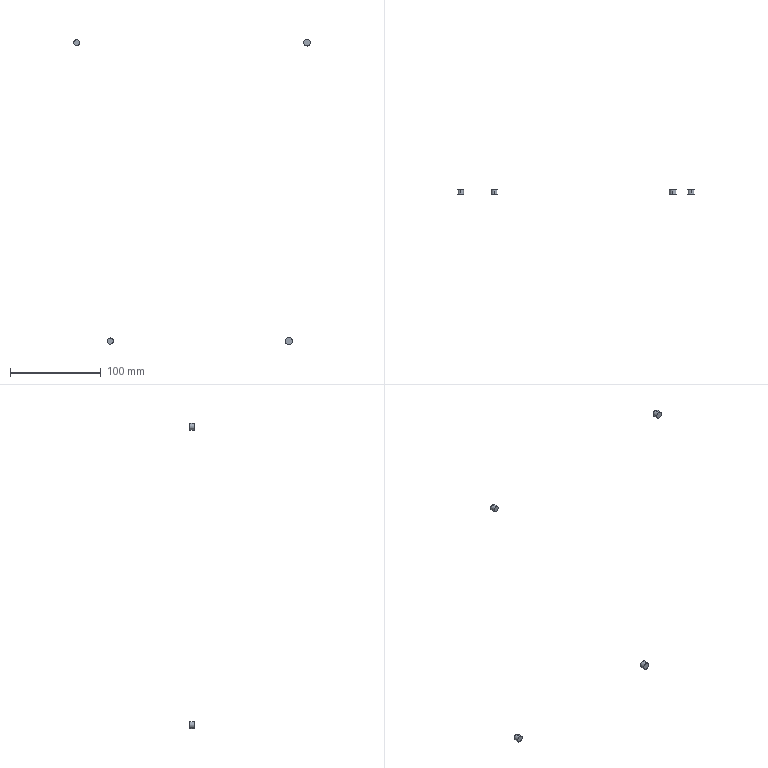Part | STEP file | Pump body | 4 solids | 16 faces | box 260.983 x 5.5 x 336.605 mm | volume 899.272 mm3 | cylinder 8 | plane 8 | commonest cylinder face diameters 6.574 x2 7.014 x2 7.393 x2 7.818 x2
STEP:
#1=CARTESIAN_POINT('',(0.,0.,0.));
#2=DIRECTION('',(0.,0.,1.));
#3=DIRECTION('',(1.,0.,0.));
#4=AXIS2_PLACEMENT_3D('',#1,#2,#3);
#5=CARTESIAN_POINT('',(105.,372.3,-20.091));
#6=VERTEX_POINT('',#5);
#7=CARTESIAN_POINT('',(105.,372.3,-27.909));
#8=VERTEX_POINT('',#7);
#9=CARTESIAN_POINT('',(105.,372.3,-24.));
#10=DIRECTION('',(0.,1.,0.));
#11=DIRECTION('',(0.,0.,1.));
#12=AXIS2_PLACEMENT_3D('',#9,#10,#11);
#13=CIRCLE('',#12,3.909);
#14=CARTESIAN_POINT('',(105.,372.3,-24.));
#15=DIRECTION('',(0.,1.,0.));
#16=DIRECTION('',(0.,0.,1.));
#17=AXIS2_PLACEMENT_3D('',#14,#15,#16);
#18=CYLINDRICAL_SURFACE('',#17,3.909);
#19=CARTESIAN_POINT('',(0.,0.));
#20=DIRECTION('',(1.,0.));
#21=VECTOR('',#20,1.);
#22=LINE('',#19,#21);
#23=(GEOMETRIC_REPRESENTATION_CONTEXT(2)PARAMETRIC_REPRESENTATION_CONTEXT()REPRESENTATION_CONTEXT('',''));
#24=DEFINITIONAL_REPRESENTATION('',(#22),#23);
#25=PCURVE('',#18,#24);
#26=CARTESIAN_POINT('',(105.,372.3,-24.));
#27=DIRECTION('',(0.,1.,0.));
#28=DIRECTION('',(0.,0.,1.));
#29=AXIS2_PLACEMENT_3D('',#26,#27,#28);
#30=PLANE('',#29);
#31=CARTESIAN_POINT('',(0.,0.));
#32=DIRECTION('',(1.,0.));
#33=AXIS2_PLACEMENT_2D('',#31,#32);
#34=CIRCLE('',#33,3.909);
#35=(GEOMETRIC_REPRESENTATION_CONTEXT(2)PARAMETRIC_REPRESENTATION_CONTEXT()REPRESENTATION_CONTEXT('',''));
#36=DEFINITIONAL_REPRESENTATION('',(#34),#35);
#37=PCURVE('',#30,#36);
#38=SURFACE_CURVE('',#13,(#25,#37),.PCURVE_S1.);
#39=EDGE_CURVE('',#6,#8,#38,.T.);
#40=ORIENTED_EDGE('',*,*,#39,.T.);
#41=CARTESIAN_POINT('',(105.,377.8,-27.909));
#42=VERTEX_POINT('',#41);
#43=CARTESIAN_POINT('',(105.,372.3,-27.909));
#44=DIRECTION('',(0.,1.,0.));
#45=VECTOR('',#44,1.);
#46=LINE('',#43,#45);
#47=CARTESIAN_POINT('',(3.142,0.));
#48=DIRECTION('',(0.,1.));
#49=VECTOR('',#48,1.);
#50=LINE('',#47,#49);
#51=(GEOMETRIC_REPRESENTATION_CONTEXT(2)PARAMETRIC_REPRESENTATION_CONTEXT()REPRESENTATION_CONTEXT('',''));
#52=DEFINITIONAL_REPRESENTATION('',(#50),#51);
#53=PCURVE('',#18,#52);
#54=CARTESIAN_POINT('',(105.,372.3,-24.));
#55=DIRECTION('',(0.,1.,0.));
#56=DIRECTION('',(0.,0.,1.));
#57=AXIS2_PLACEMENT_3D('',#54,#55,#56);
#58=CYLINDRICAL_SURFACE('',#57,3.909);
#59=CARTESIAN_POINT('',(3.142,0.));
#60=DIRECTION('',(0.,1.));
#61=VECTOR('',#60,1.);
#62=LINE('',#59,#61);
#63=(GEOMETRIC_REPRESENTATION_CONTEXT(2)PARAMETRIC_REPRESENTATION_CONTEXT()REPRESENTATION_CONTEXT('',''));
#64=DEFINITIONAL_REPRESENTATION('',(#62),#63);
#65=PCURVE('',#58,#64);
#66=SURFACE_CURVE('',#46,(#53,#65),.PCURVE_S1.);
#67=EDGE_CURVE('',#8,#42,#66,.T.);
#68=ORIENTED_EDGE('',*,*,#67,.T.);
#69=CARTESIAN_POINT('',(105.,377.8,-20.091));
#70=VERTEX_POINT('',#69);
#71=CARTESIAN_POINT('',(105.,377.8,-24.));
#72=DIRECTION('',(0.,1.,0.));
#73=DIRECTION('',(0.,0.,1.));
#74=AXIS2_PLACEMENT_3D('',#71,#72,#73);
#75=CIRCLE('',#74,3.909);
#76=CARTESIAN_POINT('',(0.,5.5));
#77=DIRECTION('',(1.,0.));
#78=VECTOR('',#77,1.);
#79=LINE('',#76,#78);
#80=(GEOMETRIC_REPRESENTATION_CONTEXT(2)PARAMETRIC_REPRESENTATION_CONTEXT()REPRESENTATION_CONTEXT('',''));
#81=DEFINITIONAL_REPRESENTATION('',(#79),#80);
#82=PCURVE('',#18,#81);
#83=CARTESIAN_POINT('',(105.,377.8,-24.));
#84=DIRECTION('',(0.,1.,0.));
#85=DIRECTION('',(0.,0.,1.));
#86=AXIS2_PLACEMENT_3D('',#83,#84,#85);
#87=PLANE('',#86);
#88=CARTESIAN_POINT('',(0.,0.));
#89=DIRECTION('',(1.,0.));
#90=AXIS2_PLACEMENT_2D('',#88,#89);
#91=CIRCLE('',#90,3.909);
#92=(GEOMETRIC_REPRESENTATION_CONTEXT(2)PARAMETRIC_REPRESENTATION_CONTEXT()REPRESENTATION_CONTEXT('',''));
#93=DEFINITIONAL_REPRESENTATION('',(#91),#92);
#94=PCURVE('',#87,#93);
#95=SURFACE_CURVE('',#75,(#82,#94),.PCURVE_S1.);
#96=EDGE_CURVE('',#70,#42,#95,.T.);
#97=ORIENTED_EDGE('',*,*,#96,.F.);
#98=CARTESIAN_POINT('',(105.,372.3,-20.091));
#99=DIRECTION('',(0.,1.,0.));
#100=VECTOR('',#99,1.);
#101=LINE('',#98,#100);
#102=CARTESIAN_POINT('',(0.,0.));
#103=DIRECTION('',(0.,1.));
#104=VECTOR('',#103,1.);
#105=LINE('',#102,#104);
#106=(GEOMETRIC_REPRESENTATION_CONTEXT(2)PARAMETRIC_REPRESENTATION_CONTEXT()REPRESENTATION_CONTEXT('',''));
#107=DEFINITIONAL_REPRESENTATION('',(#105),#106);
#108=PCURVE('',#18,#107);
#109=CARTESIAN_POINT('',(6.283,0.));
#110=DIRECTION('',(0.,1.));
#111=VECTOR('',#110,1.);
#112=LINE('',#109,#111);
#113=(GEOMETRIC_REPRESENTATION_CONTEXT(2)PARAMETRIC_REPRESENTATION_CONTEXT()REPRESENTATION_CONTEXT('',''));
#114=DEFINITIONAL_REPRESENTATION('',(#112),#113);
#115=PCURVE('',#58,#114);
#116=SURFACE_CURVE('',#101,(#108,#115),.PCURVE_S1.);
#117=EDGE_CURVE('',#6,#70,#116,.T.);
#118=ORIENTED_EDGE('',*,*,#117,.F.);
#119=EDGE_LOOP('',(#40,#68,#97,#118));
#120=FACE_BOUND('',#119,.T.);
#121=ADVANCED_FACE('',(#120),#18,.T.);
#122=ORIENTED_EDGE('',*,*,#67,.F.);
#123=CARTESIAN_POINT('',(105.,372.3,-24.));
#124=DIRECTION('',(0.,1.,0.));
#125=DIRECTION('',(0.,0.,1.));
#126=AXIS2_PLACEMENT_3D('',#123,#124,#125);
#127=CIRCLE('',#126,3.909);
#128=CARTESIAN_POINT('',(0.,0.));
#129=DIRECTION('',(1.,0.));
#130=VECTOR('',#129,1.);
#131=LINE('',#128,#130);
#132=(GEOMETRIC_REPRESENTATION_CONTEXT(2)PARAMETRIC_REPRESENTATION_CONTEXT()REPRESENTATION_CONTEXT('',''));
#133=DEFINITIONAL_REPRESENTATION('',(#131),#132);
#134=PCURVE('',#58,#133);
#135=CARTESIAN_POINT('',(0.,0.));
#136=DIRECTION('',(1.,0.));
#137=AXIS2_PLACEMENT_2D('',#135,#136);
#138=CIRCLE('',#137,3.909);
#139=(GEOMETRIC_REPRESENTATION_CONTEXT(2)PARAMETRIC_REPRESENTATION_CONTEXT()REPRESENTATION_CONTEXT('',''));
#140=DEFINITIONAL_REPRESENTATION('',(#138),#139);
#141=PCURVE('',#30,#140);
#142=SURFACE_CURVE('',#127,(#134,#141),.PCURVE_S1.);
#143=EDGE_CURVE('',#8,#6,#142,.T.);
#144=ORIENTED_EDGE('',*,*,#143,.T.);
#145=ORIENTED_EDGE('',*,*,#117,.T.);
#146=CARTESIAN_POINT('',(105.,377.8,-24.));
#147=DIRECTION('',(0.,1.,0.));
#148=DIRECTION('',(0.,0.,1.));
#149=AXIS2_PLACEMENT_3D('',#146,#147,#148);
#150=CIRCLE('',#149,3.909);
#151=CARTESIAN_POINT('',(0.,5.5));
#152=DIRECTION('',(1.,0.));
#153=VECTOR('',#152,1.);
#154=LINE('',#151,#153);
#155=(GEOMETRIC_REPRESENTATION_CONTEXT(2)PARAMETRIC_REPRESENTATION_CONTEXT()REPRESENTATION_CONTEXT('',''));
#156=DEFINITIONAL_REPRESENTATION('',(#154),#155);
#157=PCURVE('',#58,#156);
#158=CARTESIAN_POINT('',(0.,0.));
#159=DIRECTION('',(1.,0.));
#160=AXIS2_PLACEMENT_2D('',#158,#159);
#161=CIRCLE('',#160,3.909);
#162=(GEOMETRIC_REPRESENTATION_CONTEXT(2)PARAMETRIC_REPRESENTATION_CONTEXT()REPRESENTATION_CONTEXT('',''));
#163=DEFINITIONAL_REPRESENTATION('',(#161),#162);
#164=PCURVE('',#87,#163);
#165=SURFACE_CURVE('',#150,(#157,#164),.PCURVE_S1.);
#166=EDGE_CURVE('',#42,#70,#165,.T.);
#167=ORIENTED_EDGE('',*,*,#166,.F.);
#168=EDGE_LOOP('',(#122,#144,#145,#167));
#169=FACE_BOUND('',#168,.T.);
#170=ADVANCED_FACE('',(#169),#58,.T.);
#171=ORIENTED_EDGE('',*,*,#39,.F.);
#172=ORIENTED_EDGE('',*,*,#143,.F.);
#173=EDGE_LOOP('',(#171,#172));
#174=FACE_BOUND('',#173,.T.);
#175=ADVANCED_FACE('',(#174),#30,.F.);
#176=ORIENTED_EDGE('',*,*,#96,.T.);
#177=ORIENTED_EDGE('',*,*,#166,.T.);
#178=EDGE_LOOP('',(#176,#177));
#179=FACE_BOUND('',#178,.T.);
#180=ADVANCED_FACE('',(#179),#87,.T.);
#181=CLOSED_SHELL('',(#121,#170,#175,#180));
#182=MANIFOLD_SOLID_BREP('',#181);
#183=CARTESIAN_POINT('',(-92.,372.3,-20.493));
#184=VERTEX_POINT('',#183);
#185=CARTESIAN_POINT('',(-92.,372.3,-27.507));
#186=VERTEX_POINT('',#185);
#187=CARTESIAN_POINT('',(-92.,372.3,-24.));
#188=DIRECTION('',(0.,1.,0.));
#189=DIRECTION('',(0.,0.,1.));
#190=AXIS2_PLACEMENT_3D('',#187,#188,#189);
#191=CIRCLE('',#190,3.507);
#192=CARTESIAN_POINT('',(-92.,372.3,-24.));
#193=DIRECTION('',(0.,1.,0.));
#194=DIRECTION('',(0.,0.,1.));
#195=AXIS2_PLACEMENT_3D('',#192,#193,#194);
#196=CYLINDRICAL_SURFACE('',#195,3.507);
#197=CARTESIAN_POINT('',(0.,0.));
#198=DIRECTION('',(1.,0.));
#199=VECTOR('',#198,1.);
#200=LINE('',#197,#199);
#201=(GEOMETRIC_REPRESENTATION_CONTEXT(2)PARAMETRIC_REPRESENTATION_CONTEXT()REPRESENTATION_CONTEXT('',''));
#202=DEFINITIONAL_REPRESENTATION('',(#200),#201);
#203=PCURVE('',#196,#202);
#204=CARTESIAN_POINT('',(-92.,372.3,-24.));
#205=DIRECTION('',(0.,1.,0.));
#206=DIRECTION('',(0.,0.,1.));
#207=AXIS2_PLACEMENT_3D('',#204,#205,#206);
#208=PLANE('',#207);
#209=CARTESIAN_POINT('',(0.,0.));
#210=DIRECTION('',(1.,0.));
#211=AXIS2_PLACEMENT_2D('',#209,#210);
#212=CIRCLE('',#211,3.507);
#213=(GEOMETRIC_REPRESENTATION_CONTEXT(2)PARAMETRIC_REPRESENTATION_CONTEXT()REPRESENTATION_CONTEXT('',''));
#214=DEFINITIONAL_REPRESENTATION('',(#212),#213);
#215=PCURVE('',#208,#214);
#216=SURFACE_CURVE('',#191,(#203,#215),.PCURVE_S1.);
#217=EDGE_CURVE('',#184,#186,#216,.T.);
#218=ORIENTED_EDGE('',*,*,#217,.T.);
#219=CARTESIAN_POINT('',(-92.,377.8,-27.507));
#220=VERTEX_POINT('',#219);
#221=CARTESIAN_POINT('',(-92.,372.3,-27.507));
#222=DIRECTION('',(0.,1.,0.));
#223=VECTOR('',#222,1.);
#224=LINE('',#221,#223);
#225=CARTESIAN_POINT('',(3.142,0.));
#226=DIRECTION('',(0.,1.));
#227=VECTOR('',#226,1.);
#228=LINE('',#225,#227);
#229=(GEOMETRIC_REPRESENTATION_CONTEXT(2)PARAMETRIC_REPRESENTATION_CONTEXT()REPRESENTATION_CONTEXT('',''));
#230=DEFINITIONAL_REPRESENTATION('',(#228),#229);
#231=PCURVE('',#196,#230);
#232=CARTESIAN_POINT('',(-92.,372.3,-24.));
#233=DIRECTION('',(0.,1.,0.));
#234=DIRECTION('',(0.,0.,1.));
#235=AXIS2_PLACEMENT_3D('',#232,#233,#234);
#236=CYLINDRICAL_SURFACE('',#235,3.507);
#237=CARTESIAN_POINT('',(3.142,0.));
#238=DIRECTION('',(0.,1.));
#239=VECTOR('',#238,1.);
#240=LINE('',#237,#239);
#241=(GEOMETRIC_REPRESENTATION_CONTEXT(2)PARAMETRIC_REPRESENTATION_CONTEXT()REPRESENTATION_CONTEXT('',''));
#242=DEFINITIONAL_REPRESENTATION('',(#240),#241);
#243=PCURVE('',#236,#242);
#244=SURFACE_CURVE('',#224,(#231,#243),.PCURVE_S1.);
#245=EDGE_CURVE('',#186,#220,#244,.T.);
#246=ORIENTED_EDGE('',*,*,#245,.T.);
#247=CARTESIAN_POINT('',(-92.,377.8,-20.493));
#248=VERTEX_POINT('',#247);
#249=CARTESIAN_POINT('',(-92.,377.8,-24.));
#250=DIRECTION('',(0.,1.,0.));
#251=DIRECTION('',(0.,0.,1.));
#252=AXIS2_PLACEMENT_3D('',#249,#250,#251);
#253=CIRCLE('',#252,3.507);
#254=CARTESIAN_POINT('',(0.,5.5));
#255=DIRECTION('',(1.,0.));
#256=VECTOR('',#255,1.);
#257=LINE('',#254,#256);
#258=(GEOMETRIC_REPRESENTATION_CONTEXT(2)PARAMETRIC_REPRESENTATION_CONTEXT()REPRESENTATION_CONTEXT('',''));
#259=DEFINITIONAL_REPRESENTATION('',(#257),#258);
#260=PCURVE('',#196,#259);
#261=CARTESIAN_POINT('',(-92.,377.8,-24.));
#262=DIRECTION('',(0.,1.,0.));
#263=DIRECTION('',(0.,0.,1.));
#264=AXIS2_PLACEMENT_3D('',#261,#262,#263);
#265=PLANE('',#264);
#266=CARTESIAN_POINT('',(0.,0.));
#267=DIRECTION('',(1.,0.));
#268=AXIS2_PLACEMENT_2D('',#266,#267);
#269=CIRCLE('',#268,3.507);
#270=(GEOMETRIC_REPRESENTATION_CONTEXT(2)PARAMETRIC_REPRESENTATION_CONTEXT()REPRESENTATION_CONTEXT('',''));
#271=DEFINITIONAL_REPRESENTATION('',(#269),#270);
#272=PCURVE('',#265,#271);
#273=SURFACE_CURVE('',#253,(#260,#272),.PCURVE_S1.);
#274=EDGE_CURVE('',#248,#220,#273,.T.);
#275=ORIENTED_EDGE('',*,*,#274,.F.);
#276=CARTESIAN_POINT('',(-92.,372.3,-20.493));
#277=DIRECTION('',(0.,1.,0.));
#278=VECTOR('',#277,1.);
#279=LINE('',#276,#278);
#280=CARTESIAN_POINT('',(0.,0.));
#281=DIRECTION('',(0.,1.));
#282=VECTOR('',#281,1.);
#283=LINE('',#280,#282);
#284=(GEOMETRIC_REPRESENTATION_CONTEXT(2)PARAMETRIC_REPRESENTATION_CONTEXT()REPRESENTATION_CONTEXT('',''));
#285=DEFINITIONAL_REPRESENTATION('',(#283),#284);
#286=PCURVE('',#196,#285);
#287=CARTESIAN_POINT('',(6.283,0.));
#288=DIRECTION('',(0.,1.));
#289=VECTOR('',#288,1.);
#290=LINE('',#287,#289);
#291=(GEOMETRIC_REPRESENTATION_CONTEXT(2)PARAMETRIC_REPRESENTATION_CONTEXT()REPRESENTATION_CONTEXT('',''));
#292=DEFINITIONAL_REPRESENTATION('',(#290),#291);
#293=PCURVE('',#236,#292);
#294=SURFACE_CURVE('',#279,(#286,#293),.PCURVE_S1.);
#295=EDGE_CURVE('',#184,#248,#294,.T.);
#296=ORIENTED_EDGE('',*,*,#295,.F.);
#297=EDGE_LOOP('',(#218,#246,#275,#296));
#298=FACE_BOUND('',#297,.T.);
#299=ADVANCED_FACE('',(#298),#196,.T.);
#300=ORIENTED_EDGE('',*,*,#245,.F.);
#301=CARTESIAN_POINT('',(-92.,372.3,-24.));
#302=DIRECTION('',(0.,1.,0.));
#303=DIRECTION('',(0.,0.,1.));
#304=AXIS2_PLACEMENT_3D('',#301,#302,#303);
#305=CIRCLE('',#304,3.507);
#306=CARTESIAN_POINT('',(0.,0.));
#307=DIRECTION('',(1.,0.));
#308=VECTOR('',#307,1.);
#309=LINE('',#306,#308);
#310=(GEOMETRIC_REPRESENTATION_CONTEXT(2)PARAMETRIC_REPRESENTATION_CONTEXT()REPRESENTATION_CONTEXT('',''));
#311=DEFINITIONAL_REPRESENTATION('',(#309),#310);
#312=PCURVE('',#236,#311);
#313=CARTESIAN_POINT('',(0.,0.));
#314=DIRECTION('',(1.,0.));
#315=AXIS2_PLACEMENT_2D('',#313,#314);
#316=CIRCLE('',#315,3.507);
#317=(GEOMETRIC_REPRESENTATION_CONTEXT(2)PARAMETRIC_REPRESENTATION_CONTEXT()REPRESENTATION_CONTEXT('',''));
#318=DEFINITIONAL_REPRESENTATION('',(#316),#317);
#319=PCURVE('',#208,#318);
#320=SURFACE_CURVE('',#305,(#312,#319),.PCURVE_S1.);
#321=EDGE_CURVE('',#186,#184,#320,.T.);
#322=ORIENTED_EDGE('',*,*,#321,.T.);
#323=ORIENTED_EDGE('',*,*,#295,.T.);
#324=CARTESIAN_POINT('',(-92.,377.8,-24.));
#325=DIRECTION('',(0.,1.,0.));
#326=DIRECTION('',(0.,0.,1.));
#327=AXIS2_PLACEMENT_3D('',#324,#325,#326);
#328=CIRCLE('',#327,3.507);
#329=CARTESIAN_POINT('',(0.,5.5));
#330=DIRECTION('',(1.,0.));
#331=VECTOR('',#330,1.);
#332=LINE('',#329,#331);
#333=(GEOMETRIC_REPRESENTATION_CONTEXT(2)PARAMETRIC_REPRESENTATION_CONTEXT()REPRESENTATION_CONTEXT('',''));
#334=DEFINITIONAL_REPRESENTATION('',(#332),#333);
#335=PCURVE('',#236,#334);
#336=CARTESIAN_POINT('',(0.,0.));
#337=DIRECTION('',(1.,0.));
#338=AXIS2_PLACEMENT_2D('',#336,#337);
#339=CIRCLE('',#338,3.507);
#340=(GEOMETRIC_REPRESENTATION_CONTEXT(2)PARAMETRIC_REPRESENTATION_CONTEXT()REPRESENTATION_CONTEXT('',''));
#341=DEFINITIONAL_REPRESENTATION('',(#339),#340);
#342=PCURVE('',#265,#341);
#343=SURFACE_CURVE('',#328,(#335,#342),.PCURVE_S1.);
#344=EDGE_CURVE('',#220,#248,#343,.T.);
#345=ORIENTED_EDGE('',*,*,#344,.F.);
#346=EDGE_LOOP('',(#300,#322,#323,#345));
#347=FACE_BOUND('',#346,.T.);
#348=ADVANCED_FACE('',(#347),#236,.T.);
#349=ORIENTED_EDGE('',*,*,#217,.F.);
#350=ORIENTED_EDGE('',*,*,#321,.F.);
#351=EDGE_LOOP('',(#349,#350));
#352=FACE_BOUND('',#351,.T.);
#353=ADVANCED_FACE('',(#352),#208,.F.);
#354=ORIENTED_EDGE('',*,*,#274,.T.);
#355=ORIENTED_EDGE('',*,*,#344,.T.);
#356=EDGE_LOOP('',(#354,#355));
#357=FACE_BOUND('',#356,.T.);
#358=ADVANCED_FACE('',(#357),#265,.T.);
#359=CLOSED_SHELL('',(#299,#348,#353,#358));
#360=MANIFOLD_SOLID_BREP('',#359);
#361=CARTESIAN_POINT('',(-129.,372.3,308.287));
#362=VERTEX_POINT('',#361);
#363=CARTESIAN_POINT('',(-129.,372.3,301.713));
#364=VERTEX_POINT('',#363);
#365=CARTESIAN_POINT('',(-129.,372.3,305.));
#366=DIRECTION('',(0.,1.,0.));
#367=DIRECTION('',(0.,0.,1.));
#368=AXIS2_PLACEMENT_3D('',#365,#366,#367);
#369=CIRCLE('',#368,3.287);
#370=CARTESIAN_POINT('',(-129.,372.3,305.));
#371=DIRECTION('',(0.,1.,0.));
#372=DIRECTION('',(0.,0.,1.));
#373=AXIS2_PLACEMENT_3D('',#370,#371,#372);
#374=CYLINDRICAL_SURFACE('',#373,3.287);
#375=CARTESIAN_POINT('',(0.,0.));
#376=DIRECTION('',(1.,0.));
#377=VECTOR('',#376,1.);
#378=LINE('',#375,#377);
#379=(GEOMETRIC_REPRESENTATION_CONTEXT(2)PARAMETRIC_REPRESENTATION_CONTEXT()REPRESENTATION_CONTEXT('',''));
#380=DEFINITIONAL_REPRESENTATION('',(#378),#379);
#381=PCURVE('',#374,#380);
#382=CARTESIAN_POINT('',(-129.,372.3,305.));
#383=DIRECTION('',(0.,1.,0.));
#384=DIRECTION('',(0.,0.,1.));
#385=AXIS2_PLACEMENT_3D('',#382,#383,#384);
#386=PLANE('',#385);
#387=CARTESIAN_POINT('',(0.,0.));
#388=DIRECTION('',(1.,0.));
#389=AXIS2_PLACEMENT_2D('',#387,#388);
#390=CIRCLE('',#389,3.287);
#391=(GEOMETRIC_REPRESENTATION_CONTEXT(2)PARAMETRIC_REPRESENTATION_CONTEXT()REPRESENTATION_CONTEXT('',''));
#392=DEFINITIONAL_REPRESENTATION('',(#390),#391);
#393=PCURVE('',#386,#392);
#394=SURFACE_CURVE('',#369,(#381,#393),.PCURVE_S1.);
#395=EDGE_CURVE('',#362,#364,#394,.T.);
#396=ORIENTED_EDGE('',*,*,#395,.T.);
#397=CARTESIAN_POINT('',(-129.,377.8,301.713));
#398=VERTEX_POINT('',#397);
#399=CARTESIAN_POINT('',(-129.,372.3,301.713));
#400=DIRECTION('',(0.,1.,0.));
#401=VECTOR('',#400,1.);
#402=LINE('',#399,#401);
#403=CARTESIAN_POINT('',(3.142,0.));
#404=DIRECTION('',(0.,1.));
#405=VECTOR('',#404,1.);
#406=LINE('',#403,#405);
#407=(GEOMETRIC_REPRESENTATION_CONTEXT(2)PARAMETRIC_REPRESENTATION_CONTEXT()REPRESENTATION_CONTEXT('',''));
#408=DEFINITIONAL_REPRESENTATION('',(#406),#407);
#409=PCURVE('',#374,#408);
#410=CARTESIAN_POINT('',(-129.,372.3,305.));
#411=DIRECTION('',(0.,1.,0.));
#412=DIRECTION('',(0.,0.,1.));
#413=AXIS2_PLACEMENT_3D('',#410,#411,#412);
#414=CYLINDRICAL_SURFACE('',#413,3.287);
#415=CARTESIAN_POINT('',(3.142,0.));
#416=DIRECTION('',(0.,1.));
#417=VECTOR('',#416,1.);
#418=LINE('',#415,#417);
#419=(GEOMETRIC_REPRESENTATION_CONTEXT(2)PARAMETRIC_REPRESENTATION_CONTEXT()REPRESENTATION_CONTEXT('',''));
#420=DEFINITIONAL_REPRESENTATION('',(#418),#419);
#421=PCURVE('',#414,#420);
#422=SURFACE_CURVE('',#402,(#409,#421),.PCURVE_S1.);
#423=EDGE_CURVE('',#364,#398,#422,.T.);
#424=ORIENTED_EDGE('',*,*,#423,.T.);
#425=CARTESIAN_POINT('',(-129.,377.8,308.287));
#426=VERTEX_POINT('',#425);
#427=CARTESIAN_POINT('',(-129.,377.8,305.));
#428=DIRECTION('',(0.,1.,0.));
#429=DIRECTION('',(0.,0.,1.));
#430=AXIS2_PLACEMENT_3D('',#427,#428,#429);
#431=CIRCLE('',#430,3.287);
#432=CARTESIAN_POINT('',(0.,5.5));
#433=DIRECTION('',(1.,0.));
#434=VECTOR('',#433,1.);
#435=LINE('',#432,#434);
#436=(GEOMETRIC_REPRESENTATION_CONTEXT(2)PARAMETRIC_REPRESENTATION_CONTEXT()REPRESENTATION_CONTEXT('',''));
#437=DEFINITIONAL_REPRESENTATION('',(#435),#436);
#438=PCURVE('',#374,#437);
#439=CARTESIAN_POINT('',(-129.,377.8,305.));
#440=DIRECTION('',(0.,1.,0.));
#441=DIRECTION('',(0.,0.,1.));
#442=AXIS2_PLACEMENT_3D('',#439,#440,#441);
#443=PLANE('',#442);
#444=CARTESIAN_POINT('',(0.,0.));
#445=DIRECTION('',(1.,0.));
#446=AXIS2_PLACEMENT_2D('',#444,#445);
#447=CIRCLE('',#446,3.287);
#448=(GEOMETRIC_REPRESENTATION_CONTEXT(2)PARAMETRIC_REPRESENTATION_CONTEXT()REPRESENTATION_CONTEXT('',''));
#449=DEFINITIONAL_REPRESENTATION('',(#447),#448);
#450=PCURVE('',#443,#449);
#451=SURFACE_CURVE('',#431,(#438,#450),.PCURVE_S1.);
#452=EDGE_CURVE('',#426,#398,#451,.T.);
#453=ORIENTED_EDGE('',*,*,#452,.F.);
#454=CARTESIAN_POINT('',(-129.,372.3,308.287));
#455=DIRECTION('',(0.,1.,0.));
#456=VECTOR('',#455,1.);
#457=LINE('',#454,#456);
#458=CARTESIAN_POINT('',(0.,0.));
#459=DIRECTION('',(0.,1.));
#460=VECTOR('',#459,1.);
#461=LINE('',#458,#460);
#462=(GEOMETRIC_REPRESENTATION_CONTEXT(2)PARAMETRIC_REPRESENTATION_CONTEXT()REPRESENTATION_CONTEXT('',''));
#463=DEFINITIONAL_REPRESENTATION('',(#461),#462);
#464=PCURVE('',#374,#463);
#465=CARTESIAN_POINT('',(6.283,0.));
#466=DIRECTION('',(0.,1.));
#467=VECTOR('',#466,1.);
#468=LINE('',#465,#467);
#469=(GEOMETRIC_REPRESENTATION_CONTEXT(2)PARAMETRIC_REPRESENTATION_CONTEXT()REPRESENTATION_CONTEXT('',''));
#470=DEFINITIONAL_REPRESENTATION('',(#468),#469);
#471=PCURVE('',#414,#470);
#472=SURFACE_CURVE('',#457,(#464,#471),.PCURVE_S1.);
#473=EDGE_CURVE('',#362,#426,#472,.T.);
#474=ORIENTED_EDGE('',*,*,#473,.F.);
#475=EDGE_LOOP('',(#396,#424,#453,#474));
#476=FACE_BOUND('',#475,.T.);
#477=ADVANCED_FACE('',(#476),#374,.T.);
#478=ORIENTED_EDGE('',*,*,#423,.F.);
#479=CARTESIAN_POINT('',(-129.,372.3,305.));
#480=DIRECTION('',(0.,1.,0.));
#481=DIRECTION('',(0.,0.,1.));
#482=AXIS2_PLACEMENT_3D('',#479,#480,#481);
#483=CIRCLE('',#482,3.287);
#484=CARTESIAN_POINT('',(0.,0.));
#485=DIRECTION('',(1.,0.));
#486=VECTOR('',#485,1.);
#487=LINE('',#484,#486);
#488=(GEOMETRIC_REPRESENTATION_CONTEXT(2)PARAMETRIC_REPRESENTATION_CONTEXT()REPRESENTATION_CONTEXT('',''));
#489=DEFINITIONAL_REPRESENTATION('',(#487),#488);
#490=PCURVE('',#414,#489);
#491=CARTESIAN_POINT('',(0.,0.));
#492=DIRECTION('',(1.,0.));
#493=AXIS2_PLACEMENT_2D('',#491,#492);
#494=CIRCLE('',#493,3.287);
#495=(GEOMETRIC_REPRESENTATION_CONTEXT(2)PARAMETRIC_REPRESENTATION_CONTEXT()REPRESENTATION_CONTEXT('',''));
#496=DEFINITIONAL_REPRESENTATION('',(#494),#495);
#497=PCURVE('',#386,#496);
#498=SURFACE_CURVE('',#483,(#490,#497),.PCURVE_S1.);
#499=EDGE_CURVE('',#364,#362,#498,.T.);
#500=ORIENTED_EDGE('',*,*,#499,.T.);
#501=ORIENTED_EDGE('',*,*,#473,.T.);
#502=CARTESIAN_POINT('',(-129.,377.8,305.));
#503=DIRECTION('',(0.,1.,0.));
#504=DIRECTION('',(0.,0.,1.));
#505=AXIS2_PLACEMENT_3D('',#502,#503,#504);
#506=CIRCLE('',#505,3.287);
#507=CARTESIAN_POINT('',(0.,5.5));
#508=DIRECTION('',(1.,0.));
#509=VECTOR('',#508,1.);
#510=LINE('',#507,#509);
#511=(GEOMETRIC_REPRESENTATION_CONTEXT(2)PARAMETRIC_REPRESENTATION_CONTEXT()REPRESENTATION_CONTEXT('',''));
#512=DEFINITIONAL_REPRESENTATION('',(#510),#511);
#513=PCURVE('',#414,#512);
#514=CARTESIAN_POINT('',(0.,0.));
#515=DIRECTION('',(1.,0.));
#516=AXIS2_PLACEMENT_2D('',#514,#515);
#517=CIRCLE('',#516,3.287);
#518=(GEOMETRIC_REPRESENTATION_CONTEXT(2)PARAMETRIC_REPRESENTATION_CONTEXT()REPRESENTATION_CONTEXT('',''));
#519=DEFINITIONAL_REPRESENTATION('',(#517),#518);
#520=PCURVE('',#443,#519);
#521=SURFACE_CURVE('',#506,(#513,#520),.PCURVE_S1.);
#522=EDGE_CURVE('',#398,#426,#521,.T.);
#523=ORIENTED_EDGE('',*,*,#522,.F.);
#524=EDGE_LOOP('',(#478,#500,#501,#523));
#525=FACE_BOUND('',#524,.T.);
#526=ADVANCED_FACE('',(#525),#414,.T.);
#527=ORIENTED_EDGE('',*,*,#395,.F.);
#528=ORIENTED_EDGE('',*,*,#499,.F.);
#529=EDGE_LOOP('',(#527,#528));
#530=FACE_BOUND('',#529,.T.);
#531=ADVANCED_FACE('',(#530),#386,.F.);
#532=ORIENTED_EDGE('',*,*,#452,.T.);
#533=ORIENTED_EDGE('',*,*,#522,.T.);
#534=EDGE_LOOP('',(#532,#533));
#535=FACE_BOUND('',#534,.T.);
#536=ADVANCED_FACE('',(#535),#443,.T.);
#537=CLOSED_SHELL('',(#477,#526,#531,#536));
#538=MANIFOLD_SOLID_BREP('',#537);
#539=CARTESIAN_POINT('',(125.,372.3,308.696));
#540=VERTEX_POINT('',#539);
#541=CARTESIAN_POINT('',(125.,372.3,301.304));
#542=VERTEX_POINT('',#541);
#543=CARTESIAN_POINT('',(125.,372.3,305.));
#544=DIRECTION('',(0.,1.,0.));
#545=DIRECTION('',(0.,0.,1.));
#546=AXIS2_PLACEMENT_3D('',#543,#544,#545);
#547=CIRCLE('',#546,3.696);
#548=CARTESIAN_POINT('',(125.,372.3,305.));
#549=DIRECTION('',(0.,1.,0.));
#550=DIRECTION('',(0.,0.,1.));
#551=AXIS2_PLACEMENT_3D('',#548,#549,#550);
#552=CYLINDRICAL_SURFACE('',#551,3.696);
#553=CARTESIAN_POINT('',(0.,0.));
#554=DIRECTION('',(1.,0.));
#555=VECTOR('',#554,1.);
#556=LINE('',#553,#555);
#557=(GEOMETRIC_REPRESENTATION_CONTEXT(2)PARAMETRIC_REPRESENTATION_CONTEXT()REPRESENTATION_CONTEXT('',''));
#558=DEFINITIONAL_REPRESENTATION('',(#556),#557);
#559=PCURVE('',#552,#558);
#560=CARTESIAN_POINT('',(125.,372.3,305.));
#561=DIRECTION('',(0.,1.,0.));
#562=DIRECTION('',(0.,0.,1.));
#563=AXIS2_PLACEMENT_3D('',#560,#561,#562);
#564=PLANE('',#563);
#565=CARTESIAN_POINT('',(0.,0.));
#566=DIRECTION('',(1.,0.));
#567=AXIS2_PLACEMENT_2D('',#565,#566);
#568=CIRCLE('',#567,3.696);
#569=(GEOMETRIC_REPRESENTATION_CONTEXT(2)PARAMETRIC_REPRESENTATION_CONTEXT()REPRESENTATION_CONTEXT('',''));
#570=DEFINITIONAL_REPRESENTATION('',(#568),#569);
#571=PCURVE('',#564,#570);
#572=SURFACE_CURVE('',#547,(#559,#571),.PCURVE_S1.);
#573=EDGE_CURVE('',#540,#542,#572,.T.);
#574=ORIENTED_EDGE('',*,*,#573,.T.);
#575=CARTESIAN_POINT('',(125.,377.8,301.304));
#576=VERTEX_POINT('',#575);
#577=CARTESIAN_POINT('',(125.,372.3,301.304));
#578=DIRECTION('',(0.,1.,0.));
#579=VECTOR('',#578,1.);
#580=LINE('',#577,#579);
#581=CARTESIAN_POINT('',(3.142,0.));
#582=DIRECTION('',(0.,1.));
#583=VECTOR('',#582,1.);
#584=LINE('',#581,#583);
#585=(GEOMETRIC_REPRESENTATION_CONTEXT(2)PARAMETRIC_REPRESENTATION_CONTEXT()REPRESENTATION_CONTEXT('',''));
#586=DEFINITIONAL_REPRESENTATION('',(#584),#585);
#587=PCURVE('',#552,#586);
#588=CARTESIAN_POINT('',(125.,372.3,305.));
#589=DIRECTION('',(0.,1.,0.));
#590=DIRECTION('',(0.,0.,1.));
#591=AXIS2_PLACEMENT_3D('',#588,#589,#590);
#592=CYLINDRICAL_SURFACE('',#591,3.696);
#593=CARTESIAN_POINT('',(3.142,0.));
#594=DIRECTION('',(0.,1.));
#595=VECTOR('',#594,1.);
#596=LINE('',#593,#595);
#597=(GEOMETRIC_REPRESENTATION_CONTEXT(2)PARAMETRIC_REPRESENTATION_CONTEXT()REPRESENTATION_CONTEXT('',''));
#598=DEFINITIONAL_REPRESENTATION('',(#596),#597);
#599=PCURVE('',#592,#598);
#600=SURFACE_CURVE('',#580,(#587,#599),.PCURVE_S1.);
#601=EDGE_CURVE('',#542,#576,#600,.T.);
#602=ORIENTED_EDGE('',*,*,#601,.T.);
#603=CARTESIAN_POINT('',(125.,377.8,308.696));
#604=VERTEX_POINT('',#603);
#605=CARTESIAN_POINT('',(125.,377.8,305.));
#606=DIRECTION('',(0.,1.,0.));
#607=DIRECTION('',(0.,0.,1.));
#608=AXIS2_PLACEMENT_3D('',#605,#606,#607);
#609=CIRCLE('',#608,3.696);
#610=CARTESIAN_POINT('',(0.,5.5));
#611=DIRECTION('',(1.,0.));
#612=VECTOR('',#611,1.);
#613=LINE('',#610,#612);
#614=(GEOMETRIC_REPRESENTATION_CONTEXT(2)PARAMETRIC_REPRESENTATION_CONTEXT()REPRESENTATION_CONTEXT('',''));
#615=DEFINITIONAL_REPRESENTATION('',(#613),#614);
#616=PCURVE('',#552,#615);
#617=CARTESIAN_POINT('',(125.,377.8,305.));
#618=DIRECTION('',(0.,1.,0.));
#619=DIRECTION('',(0.,0.,1.));
#620=AXIS2_PLACEMENT_3D('',#617,#618,#619);
#621=PLANE('',#620);
#622=CARTESIAN_POINT('',(0.,0.));
#623=DIRECTION('',(1.,0.));
#624=AXIS2_PLACEMENT_2D('',#622,#623);
#625=CIRCLE('',#624,3.696);
#626=(GEOMETRIC_REPRESENTATION_CONTEXT(2)PARAMETRIC_REPRESENTATION_CONTEXT()REPRESENTATION_CONTEXT('',''));
#627=DEFINITIONAL_REPRESENTATION('',(#625),#626);
#628=PCURVE('',#621,#627);
#629=SURFACE_CURVE('',#609,(#616,#628),.PCURVE_S1.);
#630=EDGE_CURVE('',#604,#576,#629,.T.);
#631=ORIENTED_EDGE('',*,*,#630,.F.);
#632=CARTESIAN_POINT('',(125.,372.3,308.696));
#633=DIRECTION('',(0.,1.,0.));
#634=VECTOR('',#633,1.);
#635=LINE('',#632,#634);
#636=CARTESIAN_POINT('',(0.,0.));
#637=DIRECTION('',(0.,1.));
#638=VECTOR('',#637,1.);
#639=LINE('',#636,#638);
#640=(GEOMETRIC_REPRESENTATION_CONTEXT(2)PARAMETRIC_REPRESENTATION_CONTEXT()REPRESENTATION_CONTEXT('',''));
#641=DEFINITIONAL_REPRESENTATION('',(#639),#640);
#642=PCURVE('',#552,#641);
#643=CARTESIAN_POINT('',(6.283,0.));
#644=DIRECTION('',(0.,1.));
#645=VECTOR('',#644,1.);
#646=LINE('',#643,#645);
#647=(GEOMETRIC_REPRESENTATION_CONTEXT(2)PARAMETRIC_REPRESENTATION_CONTEXT()REPRESENTATION_CONTEXT('',''));
#648=DEFINITIONAL_REPRESENTATION('',(#646),#647);
#649=PCURVE('',#592,#648);
#650=SURFACE_CURVE('',#635,(#642,#649),.PCURVE_S1.);
#651=EDGE_CURVE('',#540,#604,#650,.T.);
#652=ORIENTED_EDGE('',*,*,#651,.F.);
#653=EDGE_LOOP('',(#574,#602,#631,#652));
#654=FACE_BOUND('',#653,.T.);
#655=ADVANCED_FACE('',(#654),#552,.T.);
#656=ORIENTED_EDGE('',*,*,#601,.F.);
#657=CARTESIAN_POINT('',(125.,372.3,305.));
#658=DIRECTION('',(0.,1.,0.));
#659=DIRECTION('',(0.,0.,1.));
#660=AXIS2_PLACEMENT_3D('',#657,#658,#659);
#661=CIRCLE('',#660,3.696);
#662=CARTESIAN_POINT('',(0.,0.));
#663=DIRECTION('',(1.,0.));
#664=VECTOR('',#663,1.);
#665=LINE('',#662,#664);
#666=(GEOMETRIC_REPRESENTATION_CONTEXT(2)PARAMETRIC_REPRESENTATION_CONTEXT()REPRESENTATION_CONTEXT('',''));
#667=DEFINITIONAL_REPRESENTATION('',(#665),#666);
#668=PCURVE('',#592,#667);
#669=CARTESIAN_POINT('',(0.,0.));
#670=DIRECTION('',(1.,0.));
#671=AXIS2_PLACEMENT_2D('',#669,#670);
#672=CIRCLE('',#671,3.696);
#673=(GEOMETRIC_REPRESENTATION_CONTEXT(2)PARAMETRIC_REPRESENTATION_CONTEXT()REPRESENTATION_CONTEXT('',''));
#674=DEFINITIONAL_REPRESENTATION('',(#672),#673);
#675=PCURVE('',#564,#674);
#676=SURFACE_CURVE('',#661,(#668,#675),.PCURVE_S1.);
#677=EDGE_CURVE('',#542,#540,#676,.T.);
#678=ORIENTED_EDGE('',*,*,#677,.T.);
#679=ORIENTED_EDGE('',*,*,#651,.T.);
#680=CARTESIAN_POINT('',(125.,377.8,305.));
#681=DIRECTION('',(0.,1.,0.));
#682=DIRECTION('',(0.,0.,1.));
#683=AXIS2_PLACEMENT_3D('',#680,#681,#682);
#684=CIRCLE('',#683,3.696);
#685=CARTESIAN_POINT('',(0.,5.5));
#686=DIRECTION('',(1.,0.));
#687=VECTOR('',#686,1.);
#688=LINE('',#685,#687);
#689=(GEOMETRIC_REPRESENTATION_CONTEXT(2)PARAMETRIC_REPRESENTATION_CONTEXT()REPRESENTATION_CONTEXT('',''));
#690=DEFINITIONAL_REPRESENTATION('',(#688),#689);
#691=PCURVE('',#592,#690);
#692=CARTESIAN_POINT('',(0.,0.));
#693=DIRECTION('',(1.,0.));
#694=AXIS2_PLACEMENT_2D('',#692,#693);
#695=CIRCLE('',#694,3.696);
#696=(GEOMETRIC_REPRESENTATION_CONTEXT(2)PARAMETRIC_REPRESENTATION_CONTEXT()REPRESENTATION_CONTEXT('',''));
#697=DEFINITIONAL_REPRESENTATION('',(#695),#696);
#698=PCURVE('',#621,#697);
#699=SURFACE_CURVE('',#684,(#691,#698),.PCURVE_S1.);
#700=EDGE_CURVE('',#576,#604,#699,.T.);
#701=ORIENTED_EDGE('',*,*,#700,.F.);
#702=EDGE_LOOP('',(#656,#678,#679,#701));
#703=FACE_BOUND('',#702,.T.);
#704=ADVANCED_FACE('',(#703),#592,.T.);
#705=ORIENTED_EDGE('',*,*,#573,.F.);
#706=ORIENTED_EDGE('',*,*,#677,.F.);
#707=EDGE_LOOP('',(#705,#706));
#708=FACE_BOUND('',#707,.T.);
#709=ADVANCED_FACE('',(#708),#564,.F.);
#710=ORIENTED_EDGE('',*,*,#630,.T.);
#711=ORIENTED_EDGE('',*,*,#700,.T.);
#712=EDGE_LOOP('',(#710,#711));
#713=FACE_BOUND('',#712,.T.);
#714=ADVANCED_FACE('',(#713),#621,.T.);
#715=CLOSED_SHELL('',(#655,#704,#709,#714));
#716=MANIFOLD_SOLID_BREP('',#715);
#717=(LENGTH_UNIT()NAMED_UNIT(*)SI_UNIT(.MILLI.,.METRE.));
#718=UNCERTAINTY_MEASURE_WITH_UNIT(LENGTH_MEASURE(0.0000001),#717,'','');
#719=(NAMED_UNIT(*)PLANE_ANGLE_UNIT()SI_UNIT($,.RADIAN.));
#720=(NAMED_UNIT(*)SI_UNIT($,.STERADIAN.)SOLID_ANGLE_UNIT());
#721=(GEOMETRIC_REPRESENTATION_CONTEXT(3)GLOBAL_UNCERTAINTY_ASSIGNED_CONTEXT((#718))GLOBAL_UNIT_ASSIGNED_CONTEXT((#717,#719,#720))REPRESENTATION_CONTEXT('',''));
#722=SHAPE_REPRESENTATION('',(#4,#182,#360,#538,#716),#721);